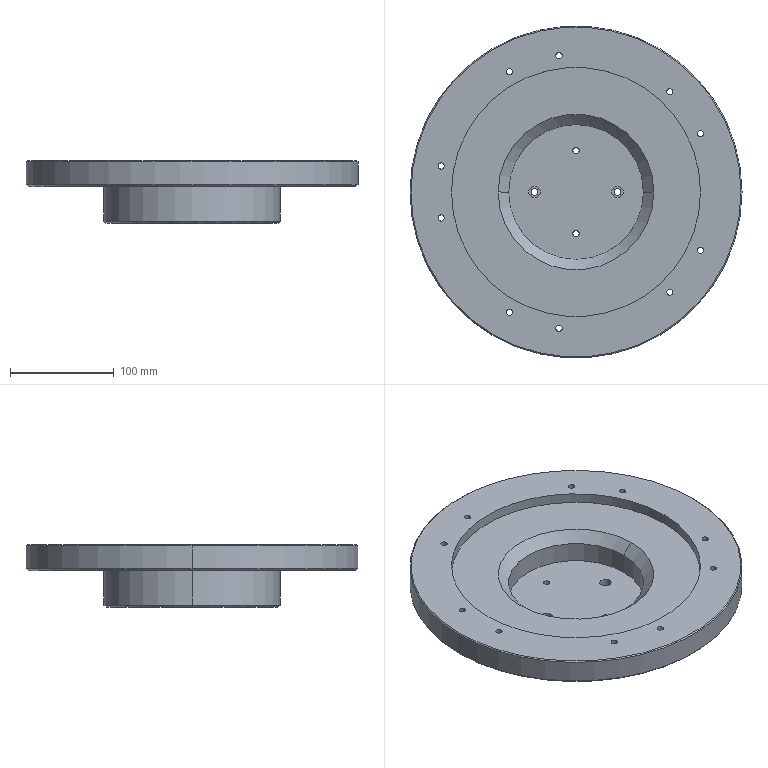NC program | NX | posted with a generic post | part box 320 x 320 x 60 mm
Lines 198 to 971 of 10816:
(ZLEVEL_PROFILE , TOOL : D20)
N394 T20 M6
N396 G54
N398 G17 G0 G90 X-163.524 Y-46.898 S7000 M3
N400 G43 Z90. H20
N402 Z61.5
N404 G94 G1 X-163.689 Y-46.368 Z61.471 F1000.
N406 X-165.857 Y-37.888 Z61.012
N408 X-167.587 Y-29.308 Z60.554
N410 X-168.872 Y-20.651 Z60.095
N412 X-169.711 Y-11.939 Z59.636
N414 X-170.1 Y-3.195 Z59.177
N416 Y0. Z59.01
N418 Y0.017 F3000.
N420 G2 X0.017 Y170.1 R170.1
N422 X-170.1 Y0. R-170.1
N424 G1 X-170.099 Y0.545 Z59.
N426 X-170.097 Y1.091 Z58.991
N428 X-170.092 Y1.636 Z58.981
N430 X-170.086 Y2.181 Z58.972
N432 X-170.078 Y2.727 Z58.962
N434 X-170.069 Y3.272 Z58.953
N436 X-170.057 Y3.817 Z58.943
N438 X-170.044 Y4.362 Z58.934
N440 X-170.029 Y4.908 Z58.924
N442 X-170.013 Y5.453 Z58.915
N444 X-169.994 Y5.998 Z58.905
N446 X-169.974 Y6.543 Z58.896
N448 X-169.952 Y7.088 Z58.886
N450 X-169.929 Y7.632 Z58.877
N452 X-169.903 Y8.177 Z58.867
N454 X-169.876 Y8.722 Z58.858
N456 X-169.847 Y9.266 Z58.848
N458 X-169.817 Y9.811 Z58.839
N460 X-169.785 Y10.355 Z58.829
N462 X-169.75 Y10.9 Z58.82
N464 X-169.715 Y11.444 Z58.81
N466 X-169.677 Y11.988 Z58.801
N468 X-169.638 Y12.532 Z58.791
N470 X-169.597 Y13.076 Z58.782
N472 X-169.554 Y13.619 Z58.772
N474 X-169.509 Y14.163 Z58.763
N476 X-169.463 Y14.706 Z58.753
N478 X-169.415 Y15.249 Z58.743
N480 X-169.365 Y15.793 Z58.734
N482 X-169.314 Y16.335 Z58.724
N484 X-169.261 Y16.878 Z58.715
N486 X-169.206 Y17.421 Z58.705
N488 X-169.149 Y17.963 Z58.696
N490 X-169.09 Y18.505 Z58.686
N492 X-169.03 Y19.047 Z58.677
N494 X-168.968 Y19.589 Z58.667
N496 X-168.905 Y20.131 Z58.658
N498 X-168.839 Y20.672 Z58.648
N500 X-168.772 Y21.214 Z58.639
N502 X-168.703 Y21.755 Z58.629
N504 X-168.633 Y22.295 Z58.62
N506 X-168.56 Y22.836 Z58.61
N508 X-168.486 Y23.376 Z58.601
N510 X-168.41 Y23.916 Z58.591
N512 X-168.333 Y24.456 Z58.582
N514 X-168.253 Y24.996 Z58.572
N516 X-168.172 Y25.535 Z58.563
N518 X-168.09 Y26.074 Z58.553
N520 X-168.005 Y26.613 Z58.544
N522 X-167.919 Y27.151 Z58.534
N524 X-167.831 Y27.689 Z58.525
N526 X-167.742 Y28.227 Z58.515
N528 X-167.65 Y28.765 Z58.505
N530 X-167.557 Y29.302 Z58.496
N532 X-167.462 Y29.839 Z58.486
N534 X-167.366 Y30.376 Z58.477
N536 X-167.268 Y30.913 Z58.467
N538 X-167.168 Y31.449 Z58.458
N540 X-167.066 Y31.984 Z58.448
N542 X-166.962 Y32.52 Z58.439
N544 X-166.857 Y33.055 Z58.429
N546 X-166.751 Y33.59 Z58.42
N548 X-166.642 Y34.124 Z58.41
N550 X-166.532 Y34.658 Z58.401
N552 X-166.42 Y35.192 Z58.391
N554 X-166.306 Y35.726 Z58.382
N556 X-166.191 Y36.259 Z58.372
N558 X-166.074 Y36.791 Z58.363
N560 X-165.955 Y37.323 Z58.353
N562 X-165.834 Y37.855 Z58.344
N564 X-165.712 Y38.387 Z58.334
N566 X-165.588 Y38.918 Z58.325
N568 X-165.462 Y39.449 Z58.315
N570 X-165.335 Y39.979 Z58.306
N572 X-165.206 Y40.509 Z58.296
N574 X-165.075 Y41.038 Z58.287
N576 X-164.943 Y41.567 Z58.277
N578 X-164.809 Y42.096 Z58.268
N580 X-164.673 Y42.624 Z58.258
N582 X-164.536 Y43.152 Z58.248
N584 X-164.396 Y43.679 Z58.239
N586 X-164.255 Y44.206 Z58.229
N588 X-164.113 Y44.732 Z58.22
N590 X-163.969 Y45.258 Z58.21
N592 X-163.823 Y45.784 Z58.201
N594 X-163.675 Y46.309 Z58.191
N596 X-163.526 Y46.833 Z58.182
N598 X-163.375 Y47.357 Z58.172
N600 X-163.222 Y47.881 Z58.163
N602 X-163.068 Y48.404 Z58.153
N604 X-162.912 Y48.926 Z58.144
N606 X-162.754 Y49.448 Z58.134
N608 X-162.595 Y49.97 Z58.125
N610 X-162.434 Y50.491 Z58.115
N612 X-162.271 Y51.012 Z58.106
N614 X-162.106 Y51.532 Z58.096
N616 X-161.94 Y52.051 Z58.087
N618 X-161.773 Y52.57 Z58.077
N620 X-161.603 Y53.088 Z58.068
N622 X-161.432 Y53.606 Z58.058
N624 X-161.26 Y54.123 Z58.049
N626 X-161.085 Y54.64 Z58.039
N628 X-160.909 Y55.156 Z58.03
N630 X-160.732 Y55.672 Z58.02
N632 G2 X-170.1 Y0. R-170.1
N634 G1 X-170.099 Y0.545 Z58.01
N636 X-170.097 Y1.091 Z58.001
N638 X-170.092 Y1.636 Z57.991
N640 X-170.086 Y2.181 Z57.982
N642 X-170.078 Y2.727 Z57.972
N644 X-170.069 Y3.272 Z57.963
N646 X-170.057 Y3.817 Z57.953
N648 X-170.044 Y4.362 Z57.944
N650 X-170.029 Y4.908 Z57.934
N652 X-170.013 Y5.453 Z57.925
N654 X-169.994 Y5.998 Z57.915
N656 X-169.974 Y6.543 Z57.906
N658 X-169.952 Y7.088 Z57.896
N660 X-169.929 Y7.632 Z57.887
N662 X-169.903 Y8.177 Z57.877
N664 X-169.876 Y8.722 Z57.868
N666 X-169.847 Y9.266 Z57.858
N668 X-169.817 Y9.811 Z57.849
N670 X-169.785 Y10.355 Z57.839
N672 X-169.75 Y10.9 Z57.83
N674 X-169.715 Y11.444 Z57.82
N676 X-169.677 Y11.988 Z57.811
N678 X-169.638 Y12.532 Z57.801
N680 X-169.597 Y13.076 Z57.792
N682 X-169.554 Y13.619 Z57.782
N684 X-169.509 Y14.163 Z57.773
N686 X-169.463 Y14.706 Z57.763
N688 X-169.415 Y15.249 Z57.753
N690 X-169.365 Y15.793 Z57.744
N692 X-169.314 Y16.335 Z57.734
N694 X-169.261 Y16.878 Z57.725
N696 X-169.206 Y17.421 Z57.715
N698 X-169.149 Y17.963 Z57.706
N700 X-169.09 Y18.505 Z57.696
N702 X-169.03 Y19.047 Z57.687
N704 X-168.968 Y19.589 Z57.677
N706 X-168.905 Y20.131 Z57.668
N708 X-168.839 Y20.672 Z57.658
N710 X-168.772 Y21.214 Z57.649
N712 X-168.703 Y21.755 Z57.639
N714 X-168.633 Y22.295 Z57.63
N716 X-168.56 Y22.836 Z57.62
N718 X-168.486 Y23.376 Z57.611
N720 X-168.41 Y23.916 Z57.601
N722 X-168.333 Y24.456 Z57.592
N724 X-168.253 Y24.996 Z57.582
N726 X-168.172 Y25.535 Z57.573
N728 X-168.09 Y26.074 Z57.563
N730 X-168.005 Y26.613 Z57.554
N732 X-167.919 Y27.151 Z57.544
N734 X-167.831 Y27.689 Z57.535
N736 X-167.742 Y28.227 Z57.525
N738 X-167.65 Y28.765 Z57.515
N740 X-167.557 Y29.302 Z57.506
N742 X-167.462 Y29.839 Z57.496
N744 X-167.366 Y30.376 Z57.487
N746 X-167.268 Y30.913 Z57.477
N748 X-167.168 Y31.449 Z57.468
N750 X-167.066 Y31.984 Z57.458
N752 X-166.962 Y32.52 Z57.449
N754 X-166.857 Y33.055 Z57.439
N756 X-166.751 Y33.59 Z57.43
N758 X-166.642 Y34.124 Z57.42
N760 X-166.532 Y34.658 Z57.411
N762 X-166.42 Y35.192 Z57.401
N764 X-166.306 Y35.726 Z57.392
N766 X-166.191 Y36.259 Z57.382
N768 X-166.074 Y36.791 Z57.373
N770 X-165.955 Y37.323 Z57.363
N772 X-165.834 Y37.855 Z57.354
N774 X-165.712 Y38.387 Z57.344
N776 X-165.588 Y38.918 Z57.335
N778 X-165.462 Y39.449 Z57.325
N780 X-165.335 Y39.979 Z57.316
N782 X-165.206 Y40.509 Z57.306
N784 X-165.075 Y41.038 Z57.297
N786 X-164.943 Y41.567 Z57.287
N788 X-164.809 Y42.096 Z57.278
N790 X-164.673 Y42.624 Z57.268
N792 X-164.536 Y43.152 Z57.258
N794 X-164.396 Y43.679 Z57.249
N796 X-164.255 Y44.206 Z57.239
N798 X-164.113 Y44.732 Z57.23
N800 X-163.969 Y45.258 Z57.22
N802 X-163.823 Y45.784 Z57.211
N804 X-163.675 Y46.309 Z57.201
N806 X-163.526 Y46.833 Z57.192
N808 X-163.375 Y47.357 Z57.182
N810 X-163.222 Y47.881 Z57.173
N812 X-163.068 Y48.404 Z57.163
N814 X-162.912 Y48.926 Z57.154
N816 X-162.754 Y49.448 Z57.144
N818 X-162.595 Y49.97 Z57.135
N820 X-162.434 Y50.491 Z57.125
N822 X-162.271 Y51.012 Z57.116
N824 X-162.106 Y51.532 Z57.106
N826 X-161.94 Y52.051 Z57.097
N828 X-161.773 Y52.57 Z57.087
N830 X-161.603 Y53.088 Z57.078
N832 X-161.432 Y53.606 Z57.068
N834 X-161.26 Y54.123 Z57.059
N836 X-161.085 Y54.64 Z57.049
N838 X-160.909 Y55.156 Z57.04
N840 X-160.732 Y55.672 Z57.03
N842 G2 X-170.1 Y0. R-170.1
N844 G1 X-170.099 Y0.545 Z57.02
N846 X-170.097 Y1.091 Z57.011
N848 X-170.092 Y1.636 Z57.001
N850 X-170.086 Y2.181 Z56.992
N852 X-170.078 Y2.727 Z56.982
N854 X-170.069 Y3.272 Z56.973
N856 X-170.057 Y3.817 Z56.963
N858 X-170.044 Y4.362 Z56.954
N860 X-170.029 Y4.908 Z56.944
N862 X-170.013 Y5.453 Z56.935
N864 X-169.994 Y5.998 Z56.925
N866 X-169.974 Y6.543 Z56.916
N868 X-169.952 Y7.088 Z56.906
N870 X-169.929 Y7.632 Z56.897
N872 X-169.903 Y8.177 Z56.887
N874 X-169.876 Y8.722 Z56.878
N876 X-169.847 Y9.266 Z56.868
N878 X-169.817 Y9.811 Z56.859
N880 X-169.785 Y10.355 Z56.849
N882 X-169.75 Y10.9 Z56.84
N884 X-169.715 Y11.444 Z56.83
N886 X-169.677 Y11.988 Z56.821
N888 X-169.638 Y12.532 Z56.811
N890 X-169.597 Y13.076 Z56.802
N892 X-169.554 Y13.619 Z56.792
N894 X-169.509 Y14.163 Z56.783
N896 X-169.463 Y14.706 Z56.773
N898 X-169.415 Y15.249 Z56.763
N900 X-169.365 Y15.793 Z56.754
N902 X-169.314 Y16.335 Z56.744
N904 X-169.261 Y16.878 Z56.735
N906 X-169.206 Y17.421 Z56.725
N908 X-169.149 Y17.963 Z56.716
N910 X-169.09 Y18.505 Z56.706
N912 X-169.03 Y19.047 Z56.697
N914 X-168.968 Y19.589 Z56.687
N916 X-168.905 Y20.131 Z56.678
N918 X-168.839 Y20.672 Z56.668
N920 X-168.772 Y21.214 Z56.659
N922 X-168.703 Y21.755 Z56.649
N924 X-168.633 Y22.295 Z56.64
N926 X-168.56 Y22.836 Z56.63
N928 X-168.486 Y23.376 Z56.621
N930 X-168.41 Y23.916 Z56.611
N932 X-168.333 Y24.456 Z56.602
N934 X-168.253 Y24.996 Z56.592
N936 X-168.172 Y25.535 Z56.583
N938 X-168.09 Y26.074 Z56.573
N940 X-168.005 Y26.613 Z56.564
N942 X-167.919 Y27.151 Z56.554
N944 X-167.831 Y27.689 Z56.545
N946 X-167.742 Y28.227 Z56.535
N948 X-167.65 Y28.765 Z56.525
N950 X-167.557 Y29.302 Z56.516
N952 X-167.462 Y29.839 Z56.506
N954 X-167.366 Y30.376 Z56.497
N956 X-167.268 Y30.913 Z56.487
N958 X-167.168 Y31.449 Z56.478
N960 X-167.066 Y31.984 Z56.468
N962 X-166.962 Y32.52 Z56.459
N964 X-166.857 Y33.055 Z56.449
N966 X-166.751 Y33.59 Z56.44
N968 X-166.642 Y34.124 Z56.43
N970 X-166.532 Y34.658 Z56.421
N972 X-166.42 Y35.192 Z56.411
N974 X-166.306 Y35.726 Z56.402
N976 X-166.191 Y36.259 Z56.392
N978 X-166.074 Y36.791 Z56.383
N980 X-165.955 Y37.323 Z56.373
N982 X-165.834 Y37.855 Z56.364
N984 X-165.712 Y38.387 Z56.354
N986 X-165.588 Y38.918 Z56.345
N988 X-165.462 Y39.449 Z56.335
N990 X-165.335 Y39.979 Z56.326
N992 X-165.206 Y40.509 Z56.316
N994 X-165.075 Y41.038 Z56.307
N996 X-164.943 Y41.567 Z56.297
N998 X-164.809 Y42.096 Z56.288
N1000 X-164.673 Y42.624 Z56.278
N1002 X-164.536 Y43.152 Z56.268
N1004 X-164.396 Y43.679 Z56.259
N1006 X-164.255 Y44.206 Z56.249
N1008 X-164.113 Y44.732 Z56.24
N1010 X-163.969 Y45.258 Z56.23
N1012 X-163.823 Y45.784 Z56.221
N1014 X-163.675 Y46.309 Z56.211
N1016 X-163.526 Y46.833 Z56.202
N1018 X-163.375 Y47.357 Z56.192
N1020 X-163.222 Y47.881 Z56.183
N1022 X-163.068 Y48.404 Z56.173
N1024 X-162.912 Y48.926 Z56.164
N1026 X-162.754 Y49.448 Z56.154
N1028 X-162.595 Y49.97 Z56.145
N1030 X-162.434 Y50.491 Z56.135
N1032 X-162.271 Y51.012 Z56.126
N1034 X-162.106 Y51.532 Z56.116
N1036 X-161.94 Y52.051 Z56.107
N1038 X-161.773 Y52.57 Z56.097
N1040 X-161.603 Y53.088 Z56.088
N1042 X-161.432 Y53.606 Z56.078
N1044 X-161.26 Y54.123 Z56.069
N1046 X-161.085 Y54.64 Z56.059
N1048 X-160.909 Y55.156 Z56.05
N1050 X-160.732 Y55.672 Z56.04
N1052 G2 X-170.1 Y0. R-170.1
N1054 G1 X-170.099 Y0.545 Z56.03
N1056 X-170.097 Y1.091 Z56.021
N1058 X-170.092 Y1.636 Z56.011
N1060 X-170.086 Y2.181 Z56.002
N1062 X-170.078 Y2.727 Z55.992
N1064 X-170.069 Y3.272 Z55.983
N1066 X-170.057 Y3.817 Z55.973
N1068 X-170.044 Y4.362 Z55.964
N1070 X-170.029 Y4.908 Z55.954
N1072 X-170.013 Y5.453 Z55.945
N1074 X-169.994 Y5.998 Z55.935
N1076 X-169.974 Y6.543 Z55.926
N1078 X-169.952 Y7.088 Z55.916
N1080 X-169.929 Y7.632 Z55.907
N1082 X-169.903 Y8.177 Z55.897
N1084 X-169.876 Y8.722 Z55.888
N1086 X-169.847 Y9.266 Z55.878
N1088 X-169.817 Y9.811 Z55.869
N1090 X-169.785 Y10.355 Z55.859
N1092 X-169.75 Y10.9 Z55.85
N1094 X-169.715 Y11.444 Z55.84
N1096 X-169.677 Y11.988 Z55.831
N1098 X-169.638 Y12.532 Z55.821
N1100 X-169.597 Y13.076 Z55.812
N1102 X-169.554 Y13.619 Z55.802
N1104 X-169.509 Y14.163 Z55.793
N1106 X-169.463 Y14.706 Z55.783
N1108 X-169.415 Y15.249 Z55.773
N1110 X-169.365 Y15.793 Z55.764
N1112 X-169.314 Y16.335 Z55.754
N1114 X-169.261 Y16.878 Z55.745
N1116 X-169.206 Y17.421 Z55.735
N1118 X-169.149 Y17.963 Z55.726
N1120 X-169.09 Y18.505 Z55.716
N1122 X-169.03 Y19.047 Z55.707
N1124 X-168.968 Y19.589 Z55.697
N1126 X-168.905 Y20.131 Z55.688
N1128 X-168.839 Y20.672 Z55.678
N1130 X-168.772 Y21.214 Z55.669
N1132 X-168.703 Y21.755 Z55.659
N1134 X-168.633 Y22.295 Z55.65
N1136 X-168.56 Y22.836 Z55.64
N1138 X-168.486 Y23.376 Z55.631
N1140 X-168.41 Y23.916 Z55.621
N1142 X-168.333 Y24.456 Z55.612
N1144 X-168.253 Y24.996 Z55.602
N1146 X-168.172 Y25.535 Z55.593
N1148 X-168.09 Y26.074 Z55.583
N1150 X-168.005 Y26.613 Z55.574
N1152 X-167.919 Y27.151 Z55.564
N1154 X-167.831 Y27.689 Z55.555
N1156 X-167.742 Y28.227 Z55.545
N1158 X-167.65 Y28.765 Z55.535
N1160 X-167.557 Y29.302 Z55.526
N1162 X-167.462 Y29.839 Z55.516
N1164 X-167.366 Y30.376 Z55.507
N1166 X-167.268 Y30.913 Z55.497
N1168 X-167.168 Y31.449 Z55.488
N1170 X-167.066 Y31.984 Z55.478
N1172 X-166.962 Y32.52 Z55.469
N1174 X-166.857 Y33.055 Z55.459
N1176 X-166.751 Y33.59 Z55.45
N1178 X-166.642 Y34.124 Z55.44
N1180 X-166.532 Y34.658 Z55.431
N1182 X-166.42 Y35.192 Z55.421
N1184 X-166.306 Y35.726 Z55.412
N1186 X-166.191 Y36.259 Z55.402
N1188 X-166.074 Y36.791 Z55.393
N1190 X-165.955 Y37.323 Z55.383
N1192 X-165.834 Y37.855 Z55.374
N1194 X-165.712 Y38.387 Z55.364
N1196 X-165.588 Y38.918 Z55.355
N1198 X-165.462 Y39.449 Z55.345
N1200 X-165.335 Y39.979 Z55.336
N1202 X-165.206 Y40.509 Z55.326
N1204 X-165.075 Y41.038 Z55.317
N1206 X-164.943 Y41.567 Z55.307
N1208 X-164.809 Y42.096 Z55.298
N1210 X-164.673 Y42.624 Z55.288
N1212 X-164.536 Y43.152 Z55.278
N1214 X-164.396 Y43.679 Z55.269
N1216 X-164.255 Y44.206 Z55.259
N1218 X-164.113 Y44.732 Z55.25
N1220 X-163.969 Y45.258 Z55.24
N1222 X-163.823 Y45.784 Z55.231
N1224 X-163.675 Y46.309 Z55.221
N1226 X-163.526 Y46.833 Z55.212
N1228 X-163.375 Y47.357 Z55.202
N1230 X-163.222 Y47.881 Z55.193
N1232 X-163.068 Y48.404 Z55.183
N1234 X-162.912 Y48.926 Z55.174
N1236 X-162.754 Y49.448 Z55.164
N1238 X-162.595 Y49.97 Z55.155
N1240 X-162.434 Y50.491 Z55.145
N1242 X-162.271 Y51.012 Z55.136
N1244 X-162.106 Y51.532 Z55.126
N1246 X-161.94 Y52.051 Z55.117
N1248 X-161.773 Y52.57 Z55.107
N1250 X-161.603 Y53.088 Z55.098
N1252 X-161.432 Y53.606 Z55.088
N1254 X-161.26 Y54.123 Z55.079
N1256 X-161.085 Y54.64 Z55.069
N1258 X-160.909 Y55.156 Z55.06
N1260 X-160.732 Y55.672 Z55.05
N1262 G2 X-170.1 Y0. R-170.1
N1264 G1 X-170.099 Y0.545 Z55.04
N1266 X-170.097 Y1.091 Z55.031
N1268 X-170.092 Y1.636 Z55.021
N1270 X-170.086 Y2.181 Z55.012
N1272 X-170.078 Y2.727 Z55.002
N1274 X-170.069 Y3.272 Z54.993
N1276 X-170.057 Y3.817 Z54.983
N1278 X-170.044 Y4.362 Z54.974
N1280 X-170.029 Y4.908 Z54.964
N1282 X-170.013 Y5.453 Z54.955
N1284 X-169.994 Y5.998 Z54.945
N1286 X-169.974 Y6.543 Z54.936
N1288 X-169.952 Y7.088 Z54.926
N1290 X-169.929 Y7.632 Z54.917
N1292 X-169.903 Y8.177 Z54.907
N1294 X-169.876 Y8.722 Z54.898
N1296 X-169.847 Y9.266 Z54.888
N1298 X-169.817 Y9.811 Z54.879
N1300 X-169.785 Y10.355 Z54.869
N1302 X-169.75 Y10.9 Z54.86
N1304 X-169.715 Y11.444 Z54.85
N1306 X-169.677 Y11.988 Z54.841
N1308 X-169.638 Y12.532 Z54.831
N1310 X-169.597 Y13.076 Z54.822
N1312 X-169.554 Y13.619 Z54.812
N1314 X-169.509 Y14.163 Z54.803
N1316 X-169.463 Y14.706 Z54.793
N1318 X-169.415 Y15.249 Z54.783
N1320 X-169.365 Y15.793 Z54.774
N1322 X-169.314 Y16.335 Z54.764
N1324 X-169.261 Y16.878 Z54.755
N1326 X-169.206 Y17.421 Z54.745
N1328 X-169.149 Y17.963 Z54.736
N1330 X-169.09 Y18.505 Z54.726
N1332 X-169.03 Y19.047 Z54.717
N1334 X-168.968 Y19.589 Z54.707
N1336 X-168.905 Y20.131 Z54.698
N1338 X-168.839 Y20.672 Z54.688
N1340 X-168.772 Y21.214 Z54.679
N1342 X-168.703 Y21.755 Z54.669
N1344 X-168.633 Y22.295 Z54.66
N1346 X-168.56 Y22.836 Z54.65
N1348 X-168.486 Y23.376 Z54.641
N1350 X-168.41 Y23.916 Z54.631
N1352 X-168.333 Y24.456 Z54.622
N1354 X-168.253 Y24.996 Z54.612
N1356 X-168.172 Y25.535 Z54.603
N1358 X-168.09 Y26.074 Z54.593
N1360 X-168.005 Y26.613 Z54.584
N1362 X-167.919 Y27.151 Z54.574
N1364 X-167.831 Y27.689 Z54.565
N1366 X-167.742 Y28.227 Z54.555
N1368 X-167.65 Y28.765 Z54.545
N1370 X-167.557 Y29.302 Z54.536
N1372 X-167.462 Y29.839 Z54.526
N1374 X-167.366 Y30.376 Z54.517
N1376 X-167.268 Y30.913 Z54.507
N1378 X-167.168 Y31.449 Z54.498
N1380 X-167.066 Y31.984 Z54.488
N1382 X-166.962 Y32.52 Z54.479
N1384 X-166.857 Y33.055 Z54.469
N1386 X-166.751 Y33.59 Z54.46
N1388 X-166.642 Y34.124 Z54.45
N1390 X-166.532 Y34.658 Z54.441
N1392 X-166.42 Y35.192 Z54.431
N1394 X-166.306 Y35.726 Z54.422
N1396 X-166.191 Y36.259 Z54.412
N1398 X-166.074 Y36.791 Z54.403
N1400 X-165.955 Y37.323 Z54.393
N1402 X-165.834 Y37.855 Z54.384
N1404 X-165.712 Y38.387 Z54.374
N1406 X-165.588 Y38.918 Z54.365
N1408 X-165.462 Y39.449 Z54.355
N1410 X-165.335 Y39.979 Z54.346
N1412 X-165.206 Y40.509 Z54.336
N1414 X-165.075 Y41.038 Z54.327
N1416 X-164.943 Y41.567 Z54.317
N1418 X-164.809 Y42.096 Z54.308
N1420 X-164.673 Y42.624 Z54.298
N1422 X-164.536 Y43.152 Z54.288
N1424 X-164.396 Y43.679 Z54.279
N1426 X-164.255 Y44.206 Z54.269
N1428 X-164.113 Y44.732 Z54.26
N1430 X-163.969 Y45.258 Z54.25
N1432 X-163.823 Y45.784 Z54.241
N1434 X-163.675 Y46.309 Z54.231
N1436 X-163.526 Y46.833 Z54.222
N1438 X-163.375 Y47.357 Z54.212
N1440 X-163.222 Y47.881 Z54.203
N1442 X-163.068 Y48.404 Z54.193
N1444 X-162.912 Y48.926 Z54.184
N1446 X-162.754 Y49.448 Z54.174
N1448 X-162.595 Y49.97 Z54.165
N1450 X-162.434 Y50.491 Z54.155
N1452 X-162.271 Y51.012 Z54.146
N1454 X-162.106 Y51.532 Z54.136
N1456 X-161.94 Y52.051 Z54.127
N1458 X-161.773 Y52.57 Z54.117
N1460 X-161.603 Y53.088 Z54.108
N1462 X-161.432 Y53.606 Z54.098
N1464 X-161.26 Y54.123 Z54.089
N1466 X-161.085 Y54.64 Z54.079
N1468 X-160.909 Y55.156 Z54.07
N1470 X-160.732 Y55.672 Z54.06
N1472 G2 X-170.1 Y0. R-170.1
N1474 G1 X-170.099 Y0.545 Z54.05
N1476 X-170.097 Y1.091 Z54.041
N1478 X-170.092 Y1.636 Z54.031
N1480 X-170.086 Y2.181 Z54.022
N1482 X-170.078 Y2.727 Z54.012
N1484 X-170.069 Y3.272 Z54.003
N1486 X-170.057 Y3.817 Z53.993
N1488 X-170.044 Y4.362 Z53.984
N1490 X-170.029 Y4.908 Z53.974
N1492 X-170.013 Y5.453 Z53.965
N1494 X-169.994 Y5.998 Z53.955
N1496 X-169.974 Y6.543 Z53.946
N1498 X-169.952 Y7.088 Z53.936
N1500 X-169.929 Y7.632 Z53.927
N1502 X-169.903 Y8.177 Z53.917
N1504 X-169.876 Y8.722 Z53.908
N1506 X-169.847 Y9.266 Z53.898
N1508 X-169.817 Y9.811 Z53.889
N1510 X-169.785 Y10.355 Z53.879
N1512 X-169.75 Y10.9 Z53.87
N1514 X-169.715 Y11.444 Z53.86
N1516 X-169.677 Y11.988 Z53.851
N1518 X-169.638 Y12.532 Z53.841
N1520 X-169.597 Y13.076 Z53.832
N1522 X-169.554 Y13.619 Z53.822
N1524 X-169.509 Y14.163 Z53.813
N1526 X-169.463 Y14.706 Z53.803
N1528 X-169.415 Y15.249 Z53.793
N1530 X-169.365 Y15.793 Z53.784
N1532 X-169.314 Y16.335 Z53.774
N1534 X-169.261 Y16.878 Z53.765
N1536 X-169.206 Y17.421 Z53.755
N1538 X-169.149 Y17.963 Z53.746
N1540 X-169.09 Y18.505 Z53.736
N1542 X-169.03 Y19.047 Z53.727
N1544 X-168.968 Y19.589 Z53.717
N1546 X-168.905 Y20.131 Z53.708
N1548 X-168.839 Y20.672 Z53.698
N1550 X-168.772 Y21.214 Z53.689
N1552 X-168.703 Y21.755 Z53.679
N1554 X-168.633 Y22.295 Z53.67
N1556 X-168.56 Y22.836 Z53.66
N1558 X-168.486 Y23.376 Z53.651
N1560 X-168.41 Y23.916 Z53.641
N1562 X-168.333 Y24.456 Z53.632
N1564 X-168.253 Y24.996 Z53.622
N1566 X-168.172 Y25.535 Z53.613
N1568 X-168.09 Y26.074 Z53.603
N1570 X-168.005 Y26.613 Z53.594
N1572 X-167.919 Y27.151 Z53.584
N1574 X-167.831 Y27.689 Z53.575
N1576 X-167.742 Y28.227 Z53.565
N1578 X-167.65 Y28.765 Z53.555
N1580 X-167.557 Y29.302 Z53.546
N1582 X-167.462 Y29.839 Z53.536
N1584 X-167.366 Y30.376 Z53.527
N1586 X-167.268 Y30.913 Z53.517
N1588 X-167.168 Y31.449 Z53.508
N1590 X-167.066 Y31.984 Z53.498
N1592 X-166.962 Y32.52 Z53.489
N1594 X-166.857 Y33.055 Z53.479
N1596 X-166.751 Y33.59 Z53.47
N1598 X-166.642 Y34.124 Z53.46
N1600 X-166.532 Y34.658 Z53.451
N1602 X-166.42 Y35.192 Z53.441
N1604 X-166.306 Y35.726 Z53.432
N1606 X-166.191 Y36.259 Z53.422
N1608 X-166.074 Y36.791 Z53.413
N1610 X-165.955 Y37.323 Z53.403
N1612 X-165.834 Y37.855 Z53.394
N1614 X-165.712 Y38.387 Z53.384
N1616 X-165.588 Y38.918 Z53.375
N1618 X-165.462 Y39.449 Z53.365
N1620 X-165.335 Y39.979 Z53.356
N1622 X-165.206 Y40.509 Z53.346
N1624 X-165.075 Y41.038 Z53.337
N1626 X-164.943 Y41.567 Z53.327
N1628 X-164.809 Y42.096 Z53.318
N1630 X-164.673 Y42.624 Z53.308
N1632 X-164.536 Y43.152 Z53.298
N1634 X-164.396 Y43.679 Z53.289
N1636 X-164.255 Y44.206 Z53.279
N1638 X-164.113 Y44.732 Z53.27
N1640 X-163.969 Y45.258 Z53.26
N1642 X-163.823 Y45.784 Z53.251
N1644 X-163.675 Y46.309 Z53.241
N1646 X-163.526 Y46.833 Z53.232
N1648 X-163.375 Y47.357 Z53.222
N1650 X-163.222 Y47.881 Z53.213
N1652 X-163.068 Y48.404 Z53.203
N1654 X-162.912 Y48.926 Z53.194
N1656 X-162.754 Y49.448 Z53.184
N1658 X-162.595 Y49.97 Z53.175
N1660 X-162.434 Y50.491 Z53.165
N1662 X-162.271 Y51.012 Z53.156
N1664 X-162.106 Y51.532 Z53.146
N1666 X-161.94 Y52.051 Z53.137
N1668 X-161.773 Y52.57 Z53.127
N1670 X-161.603 Y53.088 Z53.118
N1672 X-161.432 Y53.606 Z53.108
N1674 X-161.26 Y54.123 Z53.099
N1676 X-161.085 Y54.64 Z53.089
N1678 X-160.909 Y55.156 Z53.08
N1680 X-160.732 Y55.672 Z53.07
N1682 G2 X-170.1 Y0. R-170.1
N1684 G1 X-170.099 Y0.545 Z53.06
N1686 X-170.097 Y1.091 Z53.051
N1688 X-170.092 Y1.636 Z53.041
N1690 X-170.086 Y2.181 Z53.032
N1692 X-170.078 Y2.727 Z53.022
N1694 X-170.069 Y3.272 Z53.013
N1696 X-170.057 Y3.817 Z53.003
N1698 X-170.044 Y4.362 Z52.994
N1700 X-170.029 Y4.908 Z52.984
N1702 X-170.013 Y5.453 Z52.975
N1704 X-169.994 Y5.998 Z52.965
N1706 X-169.974 Y6.543 Z52.956
N1708 X-169.952 Y7.088 Z52.946
N1710 X-169.929 Y7.632 Z52.937
N1712 X-169.903 Y8.177 Z52.927
N1714 X-169.876 Y8.722 Z52.918
N1716 X-169.847 Y9.266 Z52.908
N1718 X-169.817 Y9.811 Z52.899
N1720 X-169.785 Y10.355 Z52.889
N1722 X-169.75 Y10.9 Z52.88
N1724 X-169.715 Y11.444 Z52.87
N1726 X-169.677 Y11.988 Z52.861
N1728 X-169.638 Y12.532 Z52.851
N1730 X-169.597 Y13.076 Z52.842
N1732 X-169.554 Y13.619 Z52.832
N1734 X-169.509 Y14.163 Z52.823
N1736 X-169.463 Y14.706 Z52.813
N1738 X-169.415 Y15.249 Z52.803
N1740 X-169.365 Y15.793 Z52.794
N1742 X-169.314 Y16.335 Z52.784
N1744 X-169.261 Y16.878 Z52.775
N1746 X-169.206 Y17.421 Z52.765
N1748 X-169.149 Y17.963 Z52.756
N1750 X-169.09 Y18.505 Z52.746
N1752 X-169.03 Y19.047 Z52.737
N1754 X-168.968 Y19.589 Z52.727
N1756 X-168.905 Y20.131 Z52.718
N1758 X-168.839 Y20.672 Z52.708
N1760 X-168.772 Y21.214 Z52.699
N1762 X-168.703 Y21.755 Z52.689
N1764 X-168.633 Y22.295 Z52.68
N1766 X-168.56 Y22.836 Z52.67
N1768 X-168.486 Y23.376 Z52.661
N1770 X-168.41 Y23.916 Z52.651
N1772 X-168.333 Y24.456 Z52.642
N1774 X-168.253 Y24.996 Z52.632
N1776 X-168.172 Y25.535 Z52.623
N1778 X-168.09 Y26.074 Z52.613
N1780 X-168.005 Y26.613 Z52.604
N1782 X-167.919 Y27.151 Z52.594
N1784 X-167.831 Y27.689 Z52.585
N1786 X-167.742 Y28.227 Z52.575
N1788 X-167.65 Y28.765 Z52.565
N1790 X-167.557 Y29.302 Z52.556
N1792 X-167.462 Y29.839 Z52.546
N1794 X-167.366 Y30.376 Z52.537
N1796 X-167.268 Y30.913 Z52.527
N1798 X-167.168 Y31.449 Z52.518
N1800 X-167.066 Y31.984 Z52.508
N1802 X-166.962 Y32.52 Z52.499
N1804 X-166.857 Y33.055 Z52.489
N1806 X-166.751 Y33.59 Z52.48
N1808 X-166.642 Y34.124 Z52.47
N1810 X-166.532 Y34.658 Z52.461
N1812 X-166.42 Y35.192 Z52.451
N1814 X-166.306 Y35.726 Z52.442
N1816 X-166.191 Y36.259 Z52.432
N1818 X-166.074 Y36.791 Z52.423
N1820 X-165.955 Y37.323 Z52.413
N1822 X-165.834 Y37.855 Z52.404
N1824 X-165.712 Y38.387 Z52.394
N1826 X-165.588 Y38.918 Z52.385
N1828 X-165.462 Y39.449 Z52.375
N1830 X-165.335 Y39.979 Z52.366
N1832 X-165.206 Y40.509 Z52.356
N1834 X-165.075 Y41.038 Z52.347
N1836 X-164.943 Y41.567 Z52.337
N1838 X-164.809 Y42.096 Z52.328
N1840 X-164.673 Y42.624 Z52.318
N1842 X-164.536 Y43.152 Z52.308
N1844 X-164.396 Y43.679 Z52.299
N1846 X-164.255 Y44.206 Z52.289
N1848 X-164.113 Y44.732 Z52.28
N1850 X-163.969 Y45.258 Z52.27
N1852 X-163.823 Y45.784 Z52.261
N1854 X-163.675 Y46.309 Z52.251
N1856 X-163.526 Y46.833 Z52.242
N1858 X-163.375 Y47.357 Z52.232
N1860 X-163.222 Y47.881 Z52.223
N1862 X-163.068 Y48.404 Z52.213
N1864 X-162.912 Y48.926 Z52.204
N1866 X-162.754 Y49.448 Z52.194
N1868 X-162.595 Y49.97 Z52.185
N1870 X-162.434 Y50.491 Z52.175
N1872 X-162.271 Y51.012 Z52.166
N1874 X-162.106 Y51.532 Z52.156
N1876 X-161.94 Y52.051 Z52.147
N1878 X-161.773 Y52.57 Z52.137
N1880 X-161.603 Y53.088 Z52.128
N1882 X-161.432 Y53.606 Z52.118
N1884 X-161.26 Y54.123 Z52.109
N1886 X-161.085 Y54.64 Z52.099
N1888 X-160.909 Y55.156 Z52.09
N1890 X-160.732 Y55.672 Z52.08
N1892 G2 X-170.1 Y0. R-170.1
N1894 G1 X-170.099 Y0.545 Z52.07
N1896 X-170.097 Y1.091 Z52.061
N1898 X-170.092 Y1.636 Z52.051
N1900 X-170.086 Y2.181 Z52.042
N1902 X-170.078 Y2.727 Z52.032
N1904 X-170.069 Y3.272 Z52.023
N1906 X-170.057 Y3.817 Z52.013
N1908 X-170.044 Y4.362 Z52.004
N1910 X-170.029 Y4.908 Z51.994
N1912 X-170.013 Y5.453 Z51.985
N1914 X-169.994 Y5.998 Z51.975
N1916 X-169.974 Y6.543 Z51.966
N1918 X-169.952 Y7.088 Z51.956
N1920 X-169.929 Y7.632 Z51.947
N1922 X-169.903 Y8.177 Z51.937
N1924 X-169.876 Y8.722 Z51.928
N1926 X-169.847 Y9.266 Z51.918
N1928 X-169.817 Y9.811 Z51.909
N1930 X-169.785 Y10.355 Z51.899
N1932 X-169.75 Y10.9 Z51.89
N1934 X-169.715 Y11.444 Z51.88